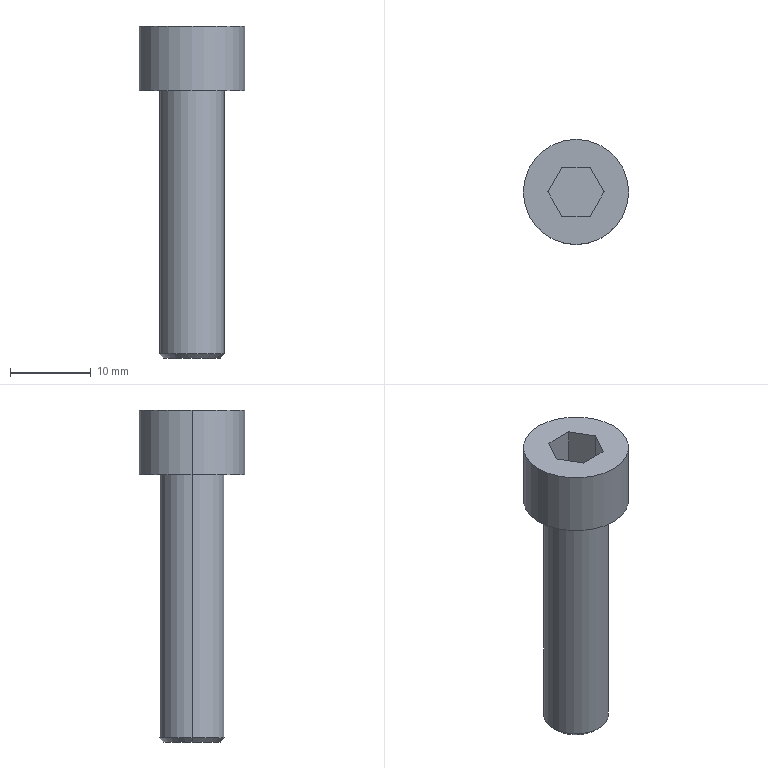Part | Creo | 1 solid | 16 faces | box 13 x 13 x 41 mm | volume 2553 mm3 | plane 10 | cylinder 4 | cone 2 | commonest cylinder face diameters 8 x2 13 x2
STEP:
#1=CARTESIAN_POINT('',(0.,0.,0.));
#2=DIRECTION('',(0.,0.,1.));
#3=DIRECTION('',(1.,0.,0.));
#4=AXIS2_PLACEMENT_3D('',#1,#2,#3);
#5=CARTESIAN_POINT('',(153.264,285.373,-70.934));
#6=VERTEX_POINT('',#5);
#7=CARTESIAN_POINT('',(161.264,285.373,-70.934));
#8=VERTEX_POINT('',#7);
#9=CARTESIAN_POINT('',(157.264,285.373,-70.934));
#10=DIRECTION('',(0.,0.,-1.));
#11=DIRECTION('',(-1.,0.,0.));
#12=AXIS2_PLACEMENT_3D('',#9,#10,#11);
#13=CIRCLE('',#12,4.);
#14=EDGE_CURVE('',#6,#8,#13,.T.);
#15=ORIENTED_EDGE('',*,*,#14,.T.);
#16=CARTESIAN_POINT('',(161.264,285.373,-38.441));
#17=VERTEX_POINT('',#16);
#18=CARTESIAN_POINT('',(161.264,285.373,-38.441));
#19=DIRECTION('',(0.,0.,-1.));
#20=VECTOR('',#19,32.493);
#21=LINE('',#18,#20);
#22=EDGE_CURVE('',#17,#8,#21,.T.);
#23=ORIENTED_EDGE('',*,*,#22,.F.);
#24=CARTESIAN_POINT('',(153.264,285.373,-38.441));
#25=VERTEX_POINT('',#24);
#26=CARTESIAN_POINT('',(157.264,285.373,-38.441));
#27=DIRECTION('',(0.,0.,1.));
#28=DIRECTION('',(1.,0.,0.));
#29=AXIS2_PLACEMENT_3D('',#26,#27,#28);
#30=CIRCLE('',#29,4.);
#31=EDGE_CURVE('',#17,#25,#30,.T.);
#32=ORIENTED_EDGE('',*,*,#31,.T.);
#33=CARTESIAN_POINT('',(153.264,285.373,-38.441));
#34=DIRECTION('',(0.,0.,-1.));
#35=VECTOR('',#34,32.493);
#36=LINE('',#33,#35);
#37=EDGE_CURVE('',#25,#6,#36,.T.);
#38=ORIENTED_EDGE('',*,*,#37,.T.);
#39=EDGE_LOOP('',(#15,#23,#32,#38));
#40=FACE_OUTER_BOUND('',#39,.F.);
#41=CARTESIAN_POINT('',(157.264,285.373,-38.441));
#42=DIRECTION('',(0.,0.,-1.));
#43=DIRECTION('',(-1.,0.,0.));
#44=AXIS2_PLACEMENT_3D('',#41,#42,#43);
#45=CYLINDRICAL_SURFACE('',#44,4.);
#46=ADVANCED_FACE('',(#40),#45,.T.);
#47=CARTESIAN_POINT('',(153.772,285.373,-71.441));
#48=VERTEX_POINT('',#47);
#49=CARTESIAN_POINT('',(160.757,285.373,-71.441));
#50=VERTEX_POINT('',#49);
#51=CARTESIAN_POINT('',(157.264,285.373,-71.441));
#52=DIRECTION('',(0.,0.,-1.));
#53=DIRECTION('',(-1.,0.,0.));
#54=AXIS2_PLACEMENT_3D('',#51,#52,#53);
#55=CIRCLE('',#54,3.493);
#56=EDGE_CURVE('',#48,#50,#55,.T.);
#57=ORIENTED_EDGE('',*,*,#56,.T.);
#58=CARTESIAN_POINT('',(160.757,285.373,-71.441));
#59=DIRECTION('',(0.7071,0.,0.7071));
#60=VECTOR('',#59,0.7176);
#61=LINE('',#58,#60);
#62=EDGE_CURVE('',#50,#8,#61,.T.);
#63=ORIENTED_EDGE('',*,*,#62,.T.);
#64=ORIENTED_EDGE('',*,*,#14,.F.);
#65=CARTESIAN_POINT('',(153.772,285.373,-71.441));
#66=DIRECTION('',(-0.7071,0.,0.7071));
#67=VECTOR('',#66,0.7176);
#68=LINE('',#65,#67);
#69=EDGE_CURVE('',#48,#6,#68,.T.);
#70=ORIENTED_EDGE('',*,*,#69,.F.);
#71=EDGE_LOOP('',(#57,#63,#64,#70));
#72=FACE_OUTER_BOUND('',#71,.F.);
#73=CARTESIAN_POINT('',(157.264,285.373,-71.188));
#74=DIRECTION('',(0.,0.,1.));
#75=DIRECTION('',(1.,0.,0.));
#76=AXIS2_PLACEMENT_3D('',#73,#74,#75);
#77=CONICAL_SURFACE('',#76,3.746,45.);
#78=ADVANCED_FACE('',(#72),#77,.T.);
#79=ORIENTED_EDGE('',*,*,#56,.F.);
#80=CARTESIAN_POINT('',(157.264,285.373,-71.441));
#81=DIRECTION('',(0.,0.,-1.));
#82=DIRECTION('',(1.,0.,0.));
#83=AXIS2_PLACEMENT_3D('',#80,#81,#82);
#84=CIRCLE('',#83,3.493);
#85=EDGE_CURVE('',#50,#48,#84,.T.);
#86=ORIENTED_EDGE('',*,*,#85,.F.);
#87=EDGE_LOOP('',(#79,#86));
#88=FACE_OUTER_BOUND('',#87,.F.);
#89=CARTESIAN_POINT('',(157.264,285.373,-71.441));
#90=DIRECTION('',(0.,0.,1.));
#91=DIRECTION('',(1.,0.,0.));
#92=AXIS2_PLACEMENT_3D('',#89,#90,#91);
#93=PLANE('',#92);
#94=ADVANCED_FACE('',(#88),#93,.F.);
#95=ORIENTED_EDGE('',*,*,#85,.T.);
#96=ORIENTED_EDGE('',*,*,#69,.T.);
#97=CARTESIAN_POINT('',(157.264,285.373,-70.934));
#98=DIRECTION('',(0.,0.,-1.));
#99=DIRECTION('',(1.,0.,0.));
#100=AXIS2_PLACEMENT_3D('',#97,#98,#99);
#101=CIRCLE('',#100,4.);
#102=EDGE_CURVE('',#8,#6,#101,.T.);
#103=ORIENTED_EDGE('',*,*,#102,.F.);
#104=ORIENTED_EDGE('',*,*,#62,.F.);
#105=EDGE_LOOP('',(#95,#96,#103,#104));
#106=FACE_OUTER_BOUND('',#105,.F.);
#107=CARTESIAN_POINT('',(157.264,285.373,-71.188));
#108=DIRECTION('',(0.,0.,1.));
#109=DIRECTION('',(1.,0.,0.));
#110=AXIS2_PLACEMENT_3D('',#107,#108,#109);
#111=CONICAL_SURFACE('',#110,3.746,45.);
#112=ADVANCED_FACE('',(#106),#111,.T.);
#113=ORIENTED_EDGE('',*,*,#102,.T.);
#114=ORIENTED_EDGE('',*,*,#37,.F.);
#115=CARTESIAN_POINT('',(157.264,285.373,-38.441));
#116=DIRECTION('',(0.,0.,1.));
#117=DIRECTION('',(-1.,0.,0.));
#118=AXIS2_PLACEMENT_3D('',#115,#116,#117);
#119=CIRCLE('',#118,4.);
#120=EDGE_CURVE('',#25,#17,#119,.T.);
#121=ORIENTED_EDGE('',*,*,#120,.T.);
#122=ORIENTED_EDGE('',*,*,#22,.T.);
#123=EDGE_LOOP('',(#113,#114,#121,#122));
#124=FACE_OUTER_BOUND('',#123,.F.);
#125=CARTESIAN_POINT('',(157.264,285.373,-38.441));
#126=DIRECTION('',(0.,0.,-1.));
#127=DIRECTION('',(-1.,0.,0.));
#128=AXIS2_PLACEMENT_3D('',#125,#126,#127);
#129=CYLINDRICAL_SURFACE('',#128,4.);
#130=ADVANCED_FACE('',(#124),#129,.T.);
#131=CARTESIAN_POINT('',(150.764,285.373,-38.441));
#132=VERTEX_POINT('',#131);
#133=CARTESIAN_POINT('',(163.764,285.373,-38.441));
#134=VERTEX_POINT('',#133);
#135=CARTESIAN_POINT('',(157.264,285.373,-38.441));
#136=DIRECTION('',(0.,0.,-1.));
#137=DIRECTION('',(-1.,0.,0.));
#138=AXIS2_PLACEMENT_3D('',#135,#136,#137);
#139=CIRCLE('',#138,6.5);
#140=EDGE_CURVE('',#132,#134,#139,.T.);
#141=ORIENTED_EDGE('',*,*,#140,.F.);
#142=CARTESIAN_POINT('',(157.264,285.373,-38.441));
#143=DIRECTION('',(0.,0.,-1.));
#144=DIRECTION('',(1.,0.,0.));
#145=AXIS2_PLACEMENT_3D('',#142,#143,#144);
#146=CIRCLE('',#145,6.5);
#147=EDGE_CURVE('',#134,#132,#146,.T.);
#148=ORIENTED_EDGE('',*,*,#147,.F.);
#149=EDGE_LOOP('',(#141,#148));
#150=FACE_OUTER_BOUND('',#149,.F.);
#151=ORIENTED_EDGE('',*,*,#120,.F.);
#152=ORIENTED_EDGE('',*,*,#31,.F.);
#153=EDGE_LOOP('',(#151,#152));
#154=FACE_BOUND('',#153,.F.);
#155=CARTESIAN_POINT('',(157.264,285.373,-38.441));
#156=DIRECTION('',(0.,0.,-1.));
#157=DIRECTION('',(-1.,0.,0.));
#158=AXIS2_PLACEMENT_3D('',#155,#156,#157);
#159=PLANE('',#158);
#160=ADVANCED_FACE('',(#150,#154),#159,.T.);
#161=CARTESIAN_POINT('',(163.764,285.373,-30.441));
#162=VERTEX_POINT('',#161);
#163=CARTESIAN_POINT('',(150.764,285.373,-30.441));
#164=VERTEX_POINT('',#163);
#165=CARTESIAN_POINT('',(157.264,285.373,-30.441));
#166=DIRECTION('',(0.,0.,1.));
#167=DIRECTION('',(1.,0.,0.));
#168=AXIS2_PLACEMENT_3D('',#165,#166,#167);
#169=CIRCLE('',#168,6.5);
#170=EDGE_CURVE('',#162,#164,#169,.T.);
#171=ORIENTED_EDGE('',*,*,#170,.T.);
#172=CARTESIAN_POINT('',(150.764,285.373,-38.441));
#173=DIRECTION('',(0.,0.,1.));
#174=VECTOR('',#173,8.);
#175=LINE('',#172,#174);
#176=EDGE_CURVE('',#132,#164,#175,.T.);
#177=ORIENTED_EDGE('',*,*,#176,.F.);
#178=ORIENTED_EDGE('',*,*,#140,.T.);
#179=CARTESIAN_POINT('',(163.764,285.373,-38.441));
#180=DIRECTION('',(0.,0.,1.));
#181=VECTOR('',#180,8.);
#182=LINE('',#179,#181);
#183=EDGE_CURVE('',#134,#162,#182,.T.);
#184=ORIENTED_EDGE('',*,*,#183,.T.);
#185=EDGE_LOOP('',(#171,#177,#178,#184));
#186=FACE_OUTER_BOUND('',#185,.F.);
#187=CARTESIAN_POINT('',(157.264,285.373,-38.441));
#188=DIRECTION('',(0.,0.,1.));
#189=DIRECTION('',(1.,0.,0.));
#190=AXIS2_PLACEMENT_3D('',#187,#188,#189);
#191=CYLINDRICAL_SURFACE('',#190,6.5);
#192=ADVANCED_FACE('',(#186),#191,.T.);
#193=CARTESIAN_POINT('',(157.264,285.373,-30.441));
#194=DIRECTION('',(0.,0.,1.));
#195=DIRECTION('',(-1.,0.,0.));
#196=AXIS2_PLACEMENT_3D('',#193,#194,#195);
#197=CIRCLE('',#196,6.5);
#198=EDGE_CURVE('',#164,#162,#197,.T.);
#199=ORIENTED_EDGE('',*,*,#198,.F.);
#200=ORIENTED_EDGE('',*,*,#170,.F.);
#201=EDGE_LOOP('',(#199,#200));
#202=FACE_OUTER_BOUND('',#201,.F.);
#203=CARTESIAN_POINT('',(155.532,288.373,-30.441));
#204=VERTEX_POINT('',#203);
#205=CARTESIAN_POINT('',(158.996,288.373,-30.441));
#206=VERTEX_POINT('',#205);
#207=CARTESIAN_POINT('',(155.532,288.373,-30.441));
#208=DIRECTION('',(1.,0.,0.));
#209=VECTOR('',#208,3.464);
#210=LINE('',#207,#209);
#211=EDGE_CURVE('',#204,#206,#210,.T.);
#212=ORIENTED_EDGE('',*,*,#211,.F.);
#213=CARTESIAN_POINT('',(153.8,285.373,-30.441));
#214=VERTEX_POINT('',#213);
#215=CARTESIAN_POINT('',(153.8,285.373,-30.441));
#216=DIRECTION('',(0.5,0.866,0.));
#217=VECTOR('',#216,3.464);
#218=LINE('',#215,#217);
#219=EDGE_CURVE('',#214,#204,#218,.T.);
#220=ORIENTED_EDGE('',*,*,#219,.F.);
#221=CARTESIAN_POINT('',(155.532,282.373,-30.441));
#222=VERTEX_POINT('',#221);
#223=CARTESIAN_POINT('',(155.532,282.373,-30.441));
#224=DIRECTION('',(-0.5,0.866,0.));
#225=VECTOR('',#224,3.464);
#226=LINE('',#223,#225);
#227=EDGE_CURVE('',#222,#214,#226,.T.);
#228=ORIENTED_EDGE('',*,*,#227,.F.);
#229=CARTESIAN_POINT('',(158.996,282.373,-30.441));
#230=VERTEX_POINT('',#229);
#231=CARTESIAN_POINT('',(158.996,282.373,-30.441));
#232=DIRECTION('',(-1.,0.,0.));
#233=VECTOR('',#232,3.464);
#234=LINE('',#231,#233);
#235=EDGE_CURVE('',#230,#222,#234,.T.);
#236=ORIENTED_EDGE('',*,*,#235,.F.);
#237=CARTESIAN_POINT('',(160.728,285.373,-30.441));
#238=VERTEX_POINT('',#237);
#239=CARTESIAN_POINT('',(160.728,285.373,-30.441));
#240=DIRECTION('',(-0.5,-0.866,0.));
#241=VECTOR('',#240,3.464);
#242=LINE('',#239,#241);
#243=EDGE_CURVE('',#238,#230,#242,.T.);
#244=ORIENTED_EDGE('',*,*,#243,.F.);
#245=CARTESIAN_POINT('',(158.996,288.373,-30.441));
#246=DIRECTION('',(0.5,-0.866,0.));
#247=VECTOR('',#246,3.464);
#248=LINE('',#245,#247);
#249=EDGE_CURVE('',#206,#238,#248,.T.);
#250=ORIENTED_EDGE('',*,*,#249,.F.);
#251=EDGE_LOOP('',(#212,#220,#228,#236,#244,#250));
#252=FACE_BOUND('',#251,.F.);
#253=CARTESIAN_POINT('',(157.264,285.373,-30.441));
#254=DIRECTION('',(0.,0.,1.));
#255=DIRECTION('',(1.,0.,0.));
#256=AXIS2_PLACEMENT_3D('',#253,#254,#255);
#257=PLANE('',#256);
#258=ADVANCED_FACE('',(#202,#252),#257,.T.);
#259=ORIENTED_EDGE('',*,*,#211,.T.);
#260=CARTESIAN_POINT('',(158.996,288.373,-35.721));
#261=VERTEX_POINT('',#260);
#262=CARTESIAN_POINT('',(158.996,288.373,-30.441));
#263=DIRECTION('',(0.,0.,-1.));
#264=VECTOR('',#263,5.28);
#265=LINE('',#262,#264);
#266=EDGE_CURVE('',#206,#261,#265,.T.);
#267=ORIENTED_EDGE('',*,*,#266,.T.);
#268=CARTESIAN_POINT('',(155.532,288.373,-35.721));
#269=VERTEX_POINT('',#268);
#270=CARTESIAN_POINT('',(155.532,288.373,-35.721));
#271=DIRECTION('',(1.,0.,0.));
#272=VECTOR('',#271,3.464);
#273=LINE('',#270,#272);
#274=EDGE_CURVE('',#269,#261,#273,.T.);
#275=ORIENTED_EDGE('',*,*,#274,.F.);
#276=CARTESIAN_POINT('',(155.532,288.373,-30.441));
#277=DIRECTION('',(0.,0.,-1.));
#278=VECTOR('',#277,5.28);
#279=LINE('',#276,#278);
#280=EDGE_CURVE('',#204,#269,#279,.T.);
#281=ORIENTED_EDGE('',*,*,#280,.F.);
#282=EDGE_LOOP('',(#259,#267,#275,#281));
#283=FACE_OUTER_BOUND('',#282,.F.);
#284=CARTESIAN_POINT('',(158.996,288.373,-35.721));
#285=DIRECTION('',(0.,1.,0.));
#286=DIRECTION('',(0.,0.,1.));
#287=AXIS2_PLACEMENT_3D('',#284,#285,#286);
#288=PLANE('',#287);
#289=ADVANCED_FACE('',(#283),#288,.F.);
#290=ORIENTED_EDGE('',*,*,#249,.T.);
#291=CARTESIAN_POINT('',(160.728,285.373,-35.721));
#292=VERTEX_POINT('',#291);
#293=CARTESIAN_POINT('',(160.728,285.373,-30.441));
#294=DIRECTION('',(0.,0.,-1.));
#295=VECTOR('',#294,5.28);
#296=LINE('',#293,#295);
#297=EDGE_CURVE('',#238,#292,#296,.T.);
#298=ORIENTED_EDGE('',*,*,#297,.T.);
#299=CARTESIAN_POINT('',(160.728,285.373,-35.721));
#300=DIRECTION('',(-0.5,0.866,0.));
#301=VECTOR('',#300,3.464);
#302=LINE('',#299,#301);
#303=EDGE_CURVE('',#292,#261,#302,.T.);
#304=ORIENTED_EDGE('',*,*,#303,.T.);
#305=ORIENTED_EDGE('',*,*,#266,.F.);
#306=EDGE_LOOP('',(#290,#298,#304,#305));
#307=FACE_OUTER_BOUND('',#306,.F.);
#308=CARTESIAN_POINT('',(160.728,285.373,-35.721));
#309=DIRECTION('',(0.866,0.5,0.));
#310=DIRECTION('',(-0.5,0.866,0.));
#311=AXIS2_PLACEMENT_3D('',#308,#309,#310);
#312=PLANE('',#311);
#313=ADVANCED_FACE('',(#307),#312,.F.);
#314=ORIENTED_EDGE('',*,*,#243,.T.);
#315=CARTESIAN_POINT('',(158.996,282.373,-35.721));
#316=VERTEX_POINT('',#315);
#317=CARTESIAN_POINT('',(158.996,282.373,-30.441));
#318=DIRECTION('',(0.,0.,-1.));
#319=VECTOR('',#318,5.28);
#320=LINE('',#317,#319);
#321=EDGE_CURVE('',#230,#316,#320,.T.);
#322=ORIENTED_EDGE('',*,*,#321,.T.);
#323=CARTESIAN_POINT('',(158.996,282.373,-35.721));
#324=DIRECTION('',(0.5,0.866,0.));
#325=VECTOR('',#324,3.464);
#326=LINE('',#323,#325);
#327=EDGE_CURVE('',#316,#292,#326,.T.);
#328=ORIENTED_EDGE('',*,*,#327,.T.);
#329=ORIENTED_EDGE('',*,*,#297,.F.);
#330=EDGE_LOOP('',(#314,#322,#328,#329));
#331=FACE_OUTER_BOUND('',#330,.F.);
#332=CARTESIAN_POINT('',(158.996,282.373,-35.721));
#333=DIRECTION('',(0.866,-0.5,0.));
#334=DIRECTION('',(0.5,0.866,0.));
#335=AXIS2_PLACEMENT_3D('',#332,#333,#334);
#336=PLANE('',#335);
#337=ADVANCED_FACE('',(#331),#336,.F.);
#338=ORIENTED_EDGE('',*,*,#235,.T.);
#339=CARTESIAN_POINT('',(155.532,282.373,-35.721));
#340=VERTEX_POINT('',#339);
#341=CARTESIAN_POINT('',(155.532,282.373,-30.441));
#342=DIRECTION('',(0.,0.,-1.));
#343=VECTOR('',#342,5.28);
#344=LINE('',#341,#343);
#345=EDGE_CURVE('',#222,#340,#344,.T.);
#346=ORIENTED_EDGE('',*,*,#345,.T.);
#347=CARTESIAN_POINT('',(158.996,282.373,-35.721));
#348=DIRECTION('',(-1.,0.,0.));
#349=VECTOR('',#348,3.464);
#350=LINE('',#347,#349);
#351=EDGE_CURVE('',#316,#340,#350,.T.);
#352=ORIENTED_EDGE('',*,*,#351,.F.);
#353=ORIENTED_EDGE('',*,*,#321,.F.);
#354=EDGE_LOOP('',(#338,#346,#352,#353));
#355=FACE_OUTER_BOUND('',#354,.F.);
#356=CARTESIAN_POINT('',(155.532,282.373,-35.721));
#357=DIRECTION('',(0.,-1.,0.));
#358=DIRECTION('',(0.,0.,-1.));
#359=AXIS2_PLACEMENT_3D('',#356,#357,#358);
#360=PLANE('',#359);
#361=ADVANCED_FACE('',(#355),#360,.F.);
#362=ORIENTED_EDGE('',*,*,#227,.T.);
#363=CARTESIAN_POINT('',(153.8,285.373,-35.721));
#364=VERTEX_POINT('',#363);
#365=CARTESIAN_POINT('',(153.8,285.373,-30.441));
#366=DIRECTION('',(0.,0.,-1.));
#367=VECTOR('',#366,5.28);
#368=LINE('',#365,#367);
#369=EDGE_CURVE('',#214,#364,#368,.T.);
#370=ORIENTED_EDGE('',*,*,#369,.T.);
#371=CARTESIAN_POINT('',(153.8,285.373,-35.721));
#372=DIRECTION('',(0.5,-0.866,0.));
#373=VECTOR('',#372,3.464);
#374=LINE('',#371,#373);
#375=EDGE_CURVE('',#364,#340,#374,.T.);
#376=ORIENTED_EDGE('',*,*,#375,.T.);
#377=ORIENTED_EDGE('',*,*,#345,.F.);
#378=EDGE_LOOP('',(#362,#370,#376,#377));
#379=FACE_OUTER_BOUND('',#378,.F.);
#380=CARTESIAN_POINT('',(153.8,285.373,-35.721));
#381=DIRECTION('',(-0.866,-0.5,0.));
#382=DIRECTION('',(0.5,-0.866,0.));
#383=AXIS2_PLACEMENT_3D('',#380,#381,#382);
#384=PLANE('',#383);
#385=ADVANCED_FACE('',(#379),#384,.F.);
#386=ORIENTED_EDGE('',*,*,#219,.T.);
#387=ORIENTED_EDGE('',*,*,#280,.T.);
#388=CARTESIAN_POINT('',(155.532,288.373,-35.721));
#389=DIRECTION('',(-0.5,-0.866,0.));
#390=VECTOR('',#389,3.464);
#391=LINE('',#388,#390);
#392=EDGE_CURVE('',#269,#364,#391,.T.);
#393=ORIENTED_EDGE('',*,*,#392,.T.);
#394=ORIENTED_EDGE('',*,*,#369,.F.);
#395=EDGE_LOOP('',(#386,#387,#393,#394));
#396=FACE_OUTER_BOUND('',#395,.F.);
#397=CARTESIAN_POINT('',(155.532,288.373,-35.721));
#398=DIRECTION('',(-0.866,0.5,0.));
#399=DIRECTION('',(-0.5,-0.866,0.));
#400=AXIS2_PLACEMENT_3D('',#397,#398,#399);
#401=PLANE('',#400);
#402=ADVANCED_FACE('',(#396),#401,.F.);
#403=ORIENTED_EDGE('',*,*,#274,.T.);
#404=ORIENTED_EDGE('',*,*,#303,.F.);
#405=ORIENTED_EDGE('',*,*,#327,.F.);
#406=ORIENTED_EDGE('',*,*,#351,.T.);
#407=ORIENTED_EDGE('',*,*,#375,.F.);
#408=ORIENTED_EDGE('',*,*,#392,.F.);
#409=EDGE_LOOP('',(#403,#404,#405,#406,#407,#408));
#410=FACE_OUTER_BOUND('',#409,.F.);
#411=CARTESIAN_POINT('',(155.532,288.373,-35.721));
#412=DIRECTION('',(0.,0.,1.));
#413=DIRECTION('',(1.,0.,0.));
#414=AXIS2_PLACEMENT_3D('',#411,#412,#413);
#415=PLANE('',#414);
#416=ADVANCED_FACE('',(#410),#415,.T.);
#417=ORIENTED_EDGE('',*,*,#198,.T.);
#418=ORIENTED_EDGE('',*,*,#183,.F.);
#419=ORIENTED_EDGE('',*,*,#147,.T.);
#420=ORIENTED_EDGE('',*,*,#176,.T.);
#421=EDGE_LOOP('',(#417,#418,#419,#420));
#422=FACE_OUTER_BOUND('',#421,.F.);
#423=CARTESIAN_POINT('',(157.264,285.373,-38.441));
#424=DIRECTION('',(0.,0.,1.));
#425=DIRECTION('',(1.,0.,0.));
#426=AXIS2_PLACEMENT_3D('',#423,#424,#425);
#427=CYLINDRICAL_SURFACE('',#426,6.5);
#428=ADVANCED_FACE('',(#422),#427,.T.);
#429=CLOSED_SHELL('',(#46,#78,#94,#112,#130,#160,#192,#258,#289,#313,#337,#361,#385,#402,#416,#428));
#430=MANIFOLD_SOLID_BREP('',#429);
#431=(LENGTH_UNIT()NAMED_UNIT(*)SI_UNIT(.MILLI.,.METRE.));
#432=UNCERTAINTY_MEASURE_WITH_UNIT(LENGTH_MEASURE(0.004494),#431,'','');
#433=(NAMED_UNIT(*)PLANE_ANGLE_UNIT()SI_UNIT($,.RADIAN.));
#434=PLANE_ANGLE_MEASURE_WITH_UNIT(PLANE_ANGLE_MEASURE(0.01745),#433);
#435=(CONVERSION_BASED_UNIT('DEGREE',#434)NAMED_UNIT(*)PLANE_ANGLE_UNIT());
#436=(NAMED_UNIT(*)SI_UNIT($,.STERADIAN.)SOLID_ANGLE_UNIT());
#437=(GEOMETRIC_REPRESENTATION_CONTEXT(3)GLOBAL_UNCERTAINTY_ASSIGNED_CONTEXT((#432))GLOBAL_UNIT_ASSIGNED_CONTEXT((#431,#435,#436))REPRESENTATION_CONTEXT('',''));
#438=ADVANCED_BREP_SHAPE_REPRESENTATION('',(#4,#430),#437);